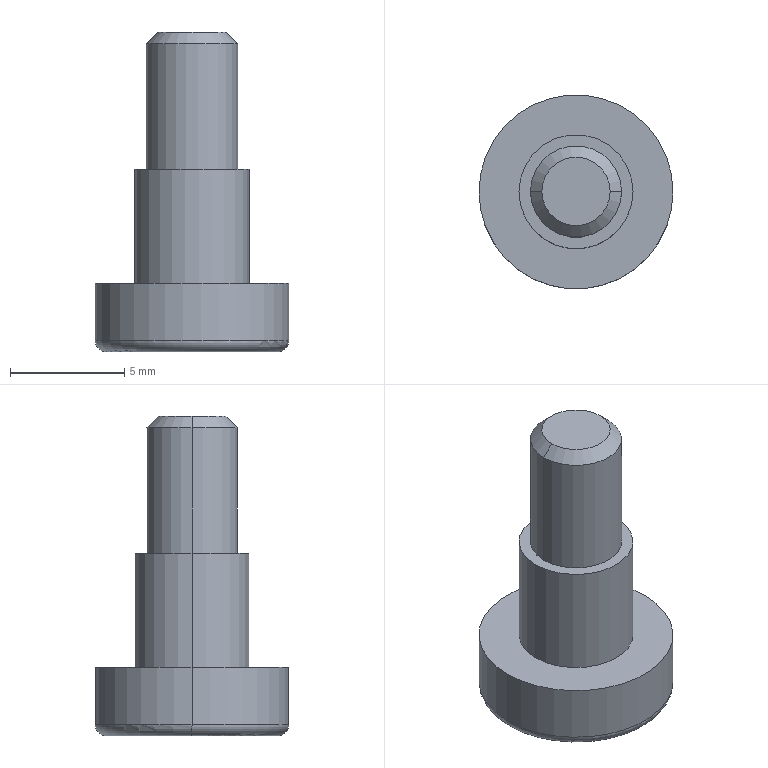Part | STEP file | 1 solid | 21 faces | box 8.5 x 8.5 x 14 mm | volume 317.59 mm3 | plane 11 | cylinder 6 | torus 2 | cone 2 | commonest cylinder face diameters 4 x2 5 x2 8.5 x2
STEP:
#1=CARTESIAN_POINT('',(0.,0.,0.));
#2=DIRECTION('',(0.,0.,1.));
#3=DIRECTION('',(1.,0.,0.));
#4=AXIS2_PLACEMENT_3D('',#1,#2,#3);
#5=CARTESIAN_POINT('',(-3.75,0.,0.));
#6=VERTEX_POINT('',#5);
#7=CARTESIAN_POINT('',(3.75,0.,0.));
#8=VERTEX_POINT('',#7);
#9=CARTESIAN_POINT('',(0.,0.,0.));
#10=DIRECTION('',(0.,0.,-1.));
#11=DIRECTION('',(1.,0.,0.));
#12=AXIS2_PLACEMENT_3D('',#9,#10,#11);
#13=CIRCLE('',#12,3.75);
#14=CARTESIAN_POINT('',(0.,0.,0.5));
#15=DIRECTION('',(0.,0.,1.));
#16=DIRECTION('',(1.,0.,0.));
#17=AXIS2_PLACEMENT_3D('',#14,#15,#16);
#18=TOROIDAL_SURFACE('',#17,3.75,0.5);
#19=CARTESIAN_POINT('',(6.283,4.712));
#20=DIRECTION('',(-1.,0.));
#21=VECTOR('',#20,1.);
#22=LINE('',#19,#21);
#23=(GEOMETRIC_REPRESENTATION_CONTEXT(2)PARAMETRIC_REPRESENTATION_CONTEXT()REPRESENTATION_CONTEXT('',''));
#24=DEFINITIONAL_REPRESENTATION('',(#22),#23);
#25=PCURVE('',#18,#24);
#26=CARTESIAN_POINT('',(0.,0.,0.));
#27=DIRECTION('',(0.,0.,1.));
#28=DIRECTION('',(1.,0.,0.));
#29=AXIS2_PLACEMENT_3D('',#26,#27,#28);
#30=PLANE('',#29);
#31=CARTESIAN_POINT('',(3.75,0.));
#32=CARTESIAN_POINT('',(3.75,-6.495));
#33=CARTESIAN_POINT('',(-1.875,-3.248));
#34=CARTESIAN_POINT('',(-7.5,0.));
#35=CARTESIAN_POINT('',(-1.875,3.248));
#36=CARTESIAN_POINT('',(3.75,6.495));
#37=CARTESIAN_POINT('',(3.75,0.));
#38=(BOUNDED_CURVE()B_SPLINE_CURVE(2,(#31,#32,#33,#34,#35,#36,#37),.UNSPECIFIED.,.T.,.F.)B_SPLINE_CURVE_WITH_KNOTS((1,2,2,2,2,1),(-2.094,0.,2.094,4.189,6.283,8.378),.UNSPECIFIED.)CURVE()GEOMETRIC_REPRESENTATION_ITEM()RATIONAL_B_SPLINE_CURVE((1.,0.5,1.,0.5,1.,0.5,1.))REPRESENTATION_ITEM(''));
#39=(GEOMETRIC_REPRESENTATION_CONTEXT(2)PARAMETRIC_REPRESENTATION_CONTEXT()REPRESENTATION_CONTEXT('',''));
#40=DEFINITIONAL_REPRESENTATION('',(#38),#39);
#41=PCURVE('',#30,#40);
#42=SURFACE_CURVE('',#13,(#25,#41),.PCURVE_S1.);
#43=EDGE_CURVE('',#6,#8,#42,.T.);
#44=ORIENTED_EDGE('',*,*,#43,.F.);
#45=CARTESIAN_POINT('',(-4.25,0.,0.5));
#46=VERTEX_POINT('',#45);
#47=CARTESIAN_POINT('',(-3.75,0.,0.5));
#48=DIRECTION('',(0.,1.,0.));
#49=DIRECTION('',(-1.,0.,0.));
#50=AXIS2_PLACEMENT_3D('',#47,#48,#49);
#51=CIRCLE('',#50,0.5);
#52=CARTESIAN_POINT('',(3.142,0.));
#53=DIRECTION('',(0.,1.));
#54=VECTOR('',#53,1.);
#55=LINE('',#52,#54);
#56=(GEOMETRIC_REPRESENTATION_CONTEXT(2)PARAMETRIC_REPRESENTATION_CONTEXT()REPRESENTATION_CONTEXT('',''));
#57=DEFINITIONAL_REPRESENTATION('',(#55),#56);
#58=PCURVE('',#18,#57);
#59=CARTESIAN_POINT('',(0.,0.,0.5));
#60=DIRECTION('',(0.,0.,1.));
#61=DIRECTION('',(1.,0.,0.));
#62=AXIS2_PLACEMENT_3D('',#59,#60,#61);
#63=TOROIDAL_SURFACE('',#62,3.75,0.5);
#64=CARTESIAN_POINT('',(3.142,0.));
#65=DIRECTION('',(0.,1.));
#66=VECTOR('',#65,1.);
#67=LINE('',#64,#66);
#68=(GEOMETRIC_REPRESENTATION_CONTEXT(2)PARAMETRIC_REPRESENTATION_CONTEXT()REPRESENTATION_CONTEXT('',''));
#69=DEFINITIONAL_REPRESENTATION('',(#67),#68);
#70=PCURVE('',#63,#69);
#71=SURFACE_CURVE('',#51,(#58,#70),.PCURVE_S1.);
#72=EDGE_CURVE('',#6,#46,#71,.T.);
#73=ORIENTED_EDGE('',*,*,#72,.T.);
#74=CARTESIAN_POINT('',(4.25,0.,0.5));
#75=VERTEX_POINT('',#74);
#76=CARTESIAN_POINT('',(0.,0.,0.5));
#77=DIRECTION('',(0.,0.,1.));
#78=DIRECTION('',(1.,0.,0.));
#79=AXIS2_PLACEMENT_3D('',#76,#77,#78);
#80=CIRCLE('',#79,4.25);
#81=CARTESIAN_POINT('',(0.,6.283));
#82=DIRECTION('',(1.,0.));
#83=VECTOR('',#82,1.);
#84=LINE('',#81,#83);
#85=(GEOMETRIC_REPRESENTATION_CONTEXT(2)PARAMETRIC_REPRESENTATION_CONTEXT()REPRESENTATION_CONTEXT('',''));
#86=DEFINITIONAL_REPRESENTATION('',(#84),#85);
#87=PCURVE('',#18,#86);
#88=CARTESIAN_POINT('',(0.,0.,3.));
#89=DIRECTION('',(0.,0.,-1.));
#90=DIRECTION('',(-1.,0.,0.));
#91=AXIS2_PLACEMENT_3D('',#88,#89,#90);
#92=CYLINDRICAL_SURFACE('',#91,4.25);
#93=CARTESIAN_POINT('',(3.142,2.5));
#94=DIRECTION('',(-1.,0.));
#95=VECTOR('',#94,1.);
#96=LINE('',#93,#95);
#97=(GEOMETRIC_REPRESENTATION_CONTEXT(2)PARAMETRIC_REPRESENTATION_CONTEXT()REPRESENTATION_CONTEXT('',''));
#98=DEFINITIONAL_REPRESENTATION('',(#96),#97);
#99=PCURVE('',#92,#98);
#100=SURFACE_CURVE('',#80,(#87,#99),.PCURVE_S1.);
#101=EDGE_CURVE('',#75,#46,#100,.T.);
#102=ORIENTED_EDGE('',*,*,#101,.F.);
#103=CARTESIAN_POINT('',(3.75,0.,0.5));
#104=DIRECTION('',(0.,-1.,0.));
#105=DIRECTION('',(0.,0.,-1.));
#106=AXIS2_PLACEMENT_3D('',#103,#104,#105);
#107=CIRCLE('',#106,0.5);
#108=CARTESIAN_POINT('',(0.,4.712));
#109=DIRECTION('',(0.,1.));
#110=VECTOR('',#109,1.);
#111=LINE('',#108,#110);
#112=(GEOMETRIC_REPRESENTATION_CONTEXT(2)PARAMETRIC_REPRESENTATION_CONTEXT()REPRESENTATION_CONTEXT('',''));
#113=DEFINITIONAL_REPRESENTATION('',(#111),#112);
#114=PCURVE('',#18,#113);
#115=CARTESIAN_POINT('',(6.283,4.712));
#116=DIRECTION('',(0.,1.));
#117=VECTOR('',#116,1.);
#118=LINE('',#115,#117);
#119=(GEOMETRIC_REPRESENTATION_CONTEXT(2)PARAMETRIC_REPRESENTATION_CONTEXT()REPRESENTATION_CONTEXT('',''));
#120=DEFINITIONAL_REPRESENTATION('',(#118),#119);
#121=PCURVE('',#63,#120);
#122=SURFACE_CURVE('',#107,(#114,#121),.PCURVE_S1.);
#123=EDGE_CURVE('',#8,#75,#122,.T.);
#124=ORIENTED_EDGE('',*,*,#123,.F.);
#125=EDGE_LOOP('',(#44,#73,#102,#124));
#126=FACE_BOUND('',#125,.T.);
#127=ADVANCED_FACE('',(#126),#18,.T.);
#128=CARTESIAN_POINT('',(1.5,0.,14.));
#129=VERTEX_POINT('',#128);
#130=CARTESIAN_POINT('',(-1.5,0.,14.));
#131=VERTEX_POINT('',#130);
#132=CARTESIAN_POINT('',(0.,0.,14.));
#133=DIRECTION('',(0.,0.,1.));
#134=DIRECTION('',(1.,0.,0.));
#135=AXIS2_PLACEMENT_3D('',#132,#133,#134);
#136=CIRCLE('',#135,1.5);
#137=CARTESIAN_POINT('',(0.,0.,14.));
#138=DIRECTION('',(0.,0.,-1.));
#139=DIRECTION('',(-1.,0.,0.));
#140=AXIS2_PLACEMENT_3D('',#137,#138,#139);
#141=CONICAL_SURFACE('',#140,1.5,0.7854);
#142=CARTESIAN_POINT('',(3.142,0.));
#143=DIRECTION('',(-1.,0.));
#144=VECTOR('',#143,1.);
#145=LINE('',#142,#144);
#146=(GEOMETRIC_REPRESENTATION_CONTEXT(2)PARAMETRIC_REPRESENTATION_CONTEXT()REPRESENTATION_CONTEXT('',''));
#147=DEFINITIONAL_REPRESENTATION('',(#145),#146);
#148=PCURVE('',#141,#147);
#149=CARTESIAN_POINT('',(0.,0.,14.));
#150=DIRECTION('',(0.,0.,1.));
#151=DIRECTION('',(1.,0.,0.));
#152=AXIS2_PLACEMENT_3D('',#149,#150,#151);
#153=PLANE('',#152);
#154=CARTESIAN_POINT('',(0.,0.));
#155=DIRECTION('',(1.,0.));
#156=AXIS2_PLACEMENT_2D('',#154,#155);
#157=CIRCLE('',#156,1.5);
#158=(GEOMETRIC_REPRESENTATION_CONTEXT(2)PARAMETRIC_REPRESENTATION_CONTEXT()REPRESENTATION_CONTEXT('',''));
#159=DEFINITIONAL_REPRESENTATION('',(#157),#158);
#160=PCURVE('',#153,#159);
#161=SURFACE_CURVE('',#136,(#148,#160),.PCURVE_S1.);
#162=EDGE_CURVE('',#129,#131,#161,.T.);
#163=ORIENTED_EDGE('',*,*,#162,.F.);
#164=CARTESIAN_POINT('',(2.,0.,13.5));
#165=VERTEX_POINT('',#164);
#166=CARTESIAN_POINT('',(1.5,0.,14.));
#167=DIRECTION('',(0.7071,0.,-0.7071));
#168=VECTOR('',#167,1.);
#169=LINE('',#166,#168);
#170=CARTESIAN_POINT('',(3.142,0.));
#171=DIRECTION('',(0.,1.));
#172=VECTOR('',#171,1.);
#173=LINE('',#170,#172);
#174=(GEOMETRIC_REPRESENTATION_CONTEXT(2)PARAMETRIC_REPRESENTATION_CONTEXT()REPRESENTATION_CONTEXT('',''));
#175=DEFINITIONAL_REPRESENTATION('',(#173),#174);
#176=PCURVE('',#141,#175);
#177=CARTESIAN_POINT('',(0.,0.,14.));
#178=DIRECTION('',(0.,0.,-1.));
#179=DIRECTION('',(-1.,0.,0.));
#180=AXIS2_PLACEMENT_3D('',#177,#178,#179);
#181=CONICAL_SURFACE('',#180,1.5,0.7854);
#182=CARTESIAN_POINT('',(3.142,0.));
#183=DIRECTION('',(0.,1.));
#184=VECTOR('',#183,1.);
#185=LINE('',#182,#184);
#186=(GEOMETRIC_REPRESENTATION_CONTEXT(2)PARAMETRIC_REPRESENTATION_CONTEXT()REPRESENTATION_CONTEXT('',''));
#187=DEFINITIONAL_REPRESENTATION('',(#185),#186);
#188=PCURVE('',#181,#187);
#189=SURFACE_CURVE('',#169,(#176,#188),.PCURVE_S1.);
#190=EDGE_CURVE('',#129,#165,#189,.T.);
#191=ORIENTED_EDGE('',*,*,#190,.T.);
#192=CARTESIAN_POINT('',(-2.,0.,13.5));
#193=VERTEX_POINT('',#192);
#194=CARTESIAN_POINT('',(0.,0.,13.5));
#195=DIRECTION('',(0.,0.,-1.));
#196=DIRECTION('',(1.,0.,0.));
#197=AXIS2_PLACEMENT_3D('',#194,#195,#196);
#198=CIRCLE('',#197,2.);
#199=CARTESIAN_POINT('',(-3.142,0.5));
#200=DIRECTION('',(1.,0.));
#201=VECTOR('',#200,1.);
#202=LINE('',#199,#201);
#203=(GEOMETRIC_REPRESENTATION_CONTEXT(2)PARAMETRIC_REPRESENTATION_CONTEXT()REPRESENTATION_CONTEXT('',''));
#204=DEFINITIONAL_REPRESENTATION('',(#202),#203);
#205=PCURVE('',#141,#204);
#206=CARTESIAN_POINT('',(0.,0.,14.));
#207=DIRECTION('',(0.,0.,-1.));
#208=DIRECTION('',(-1.,0.,0.));
#209=AXIS2_PLACEMENT_3D('',#206,#207,#208);
#210=CYLINDRICAL_SURFACE('',#209,2.);
#211=CARTESIAN_POINT('',(-3.142,0.5));
#212=DIRECTION('',(1.,0.));
#213=VECTOR('',#212,1.);
#214=LINE('',#211,#213);
#215=(GEOMETRIC_REPRESENTATION_CONTEXT(2)PARAMETRIC_REPRESENTATION_CONTEXT()REPRESENTATION_CONTEXT('',''));
#216=DEFINITIONAL_REPRESENTATION('',(#214),#215);
#217=PCURVE('',#210,#216);
#218=SURFACE_CURVE('',#198,(#205,#217),.PCURVE_S1.);
#219=EDGE_CURVE('',#193,#165,#218,.T.);
#220=ORIENTED_EDGE('',*,*,#219,.F.);
#221=CARTESIAN_POINT('',(-1.5,0.,14.));
#222=DIRECTION('',(-0.7071,0.,-0.7071));
#223=VECTOR('',#222,1.);
#224=LINE('',#221,#223);
#225=CARTESIAN_POINT('',(0.,0.));
#226=DIRECTION('',(0.,1.));
#227=VECTOR('',#226,1.);
#228=LINE('',#225,#227);
#229=(GEOMETRIC_REPRESENTATION_CONTEXT(2)PARAMETRIC_REPRESENTATION_CONTEXT()REPRESENTATION_CONTEXT('',''));
#230=DEFINITIONAL_REPRESENTATION('',(#228),#229);
#231=PCURVE('',#141,#230);
#232=CARTESIAN_POINT('',(6.283,0.));
#233=DIRECTION('',(0.,1.));
#234=VECTOR('',#233,1.);
#235=LINE('',#232,#234);
#236=(GEOMETRIC_REPRESENTATION_CONTEXT(2)PARAMETRIC_REPRESENTATION_CONTEXT()REPRESENTATION_CONTEXT('',''));
#237=DEFINITIONAL_REPRESENTATION('',(#235),#236);
#238=PCURVE('',#181,#237);
#239=SURFACE_CURVE('',#224,(#231,#238),.PCURVE_S1.);
#240=EDGE_CURVE('',#131,#193,#239,.T.);
#241=ORIENTED_EDGE('',*,*,#240,.F.);
#242=EDGE_LOOP('',(#163,#191,#220,#241));
#243=FACE_BOUND('',#242,.T.);
#244=ADVANCED_FACE('',(#243),#141,.T.);
#245=ORIENTED_EDGE('',*,*,#219,.T.);
#246=CARTESIAN_POINT('',(2.,0.,8.));
#247=VERTEX_POINT('',#246);
#248=CARTESIAN_POINT('',(2.,0.,14.));
#249=DIRECTION('',(0.,0.,-1.));
#250=VECTOR('',#249,1.);
#251=LINE('',#248,#250);
#252=CARTESIAN_POINT('',(3.142,0.));
#253=DIRECTION('',(0.,1.));
#254=VECTOR('',#253,1.);
#255=LINE('',#252,#254);
#256=(GEOMETRIC_REPRESENTATION_CONTEXT(2)PARAMETRIC_REPRESENTATION_CONTEXT()REPRESENTATION_CONTEXT('',''));
#257=DEFINITIONAL_REPRESENTATION('',(#255),#256);
#258=PCURVE('',#210,#257);
#259=CARTESIAN_POINT('',(0.,0.,14.));
#260=DIRECTION('',(0.,0.,-1.));
#261=DIRECTION('',(-1.,0.,0.));
#262=AXIS2_PLACEMENT_3D('',#259,#260,#261);
#263=CYLINDRICAL_SURFACE('',#262,2.);
#264=CARTESIAN_POINT('',(3.142,0.));
#265=DIRECTION('',(0.,1.));
#266=VECTOR('',#265,1.);
#267=LINE('',#264,#266);
#268=(GEOMETRIC_REPRESENTATION_CONTEXT(2)PARAMETRIC_REPRESENTATION_CONTEXT()REPRESENTATION_CONTEXT('',''));
#269=DEFINITIONAL_REPRESENTATION('',(#267),#268);
#270=PCURVE('',#263,#269);
#271=SURFACE_CURVE('',#251,(#258,#270),.PCURVE_S1.);
#272=EDGE_CURVE('',#165,#247,#271,.T.);
#273=ORIENTED_EDGE('',*,*,#272,.T.);
#274=CARTESIAN_POINT('',(-2.,0.,8.));
#275=VERTEX_POINT('',#274);
#276=CARTESIAN_POINT('',(0.,0.,8.));
#277=DIRECTION('',(0.,0.,1.));
#278=DIRECTION('',(1.,0.,0.));
#279=AXIS2_PLACEMENT_3D('',#276,#277,#278);
#280=CIRCLE('',#279,2.);
#281=CARTESIAN_POINT('',(3.142,6.));
#282=DIRECTION('',(-1.,0.));
#283=VECTOR('',#282,1.);
#284=LINE('',#281,#283);
#285=(GEOMETRIC_REPRESENTATION_CONTEXT(2)PARAMETRIC_REPRESENTATION_CONTEXT()REPRESENTATION_CONTEXT('',''));
#286=DEFINITIONAL_REPRESENTATION('',(#284),#285);
#287=PCURVE('',#210,#286);
#288=CARTESIAN_POINT('',(0.,0.,8.));
#289=DIRECTION('',(0.,0.,1.));
#290=DIRECTION('',(1.,0.,0.));
#291=AXIS2_PLACEMENT_3D('',#288,#289,#290);
#292=PLANE('',#291);
#293=CARTESIAN_POINT('',(0.,0.));
#294=DIRECTION('',(1.,0.));
#295=AXIS2_PLACEMENT_2D('',#293,#294);
#296=CIRCLE('',#295,2.);
#297=(GEOMETRIC_REPRESENTATION_CONTEXT(2)PARAMETRIC_REPRESENTATION_CONTEXT()REPRESENTATION_CONTEXT('',''));
#298=DEFINITIONAL_REPRESENTATION('',(#296),#297);
#299=PCURVE('',#292,#298);
#300=SURFACE_CURVE('',#280,(#287,#299),.PCURVE_S1.);
#301=EDGE_CURVE('',#247,#275,#300,.T.);
#302=ORIENTED_EDGE('',*,*,#301,.T.);
#303=CARTESIAN_POINT('',(-2.,0.,14.));
#304=DIRECTION('',(0.,0.,-1.));
#305=VECTOR('',#304,1.);
#306=LINE('',#303,#305);
#307=CARTESIAN_POINT('',(0.,0.));
#308=DIRECTION('',(0.,1.));
#309=VECTOR('',#308,1.);
#310=LINE('',#307,#309);
#311=(GEOMETRIC_REPRESENTATION_CONTEXT(2)PARAMETRIC_REPRESENTATION_CONTEXT()REPRESENTATION_CONTEXT('',''));
#312=DEFINITIONAL_REPRESENTATION('',(#310),#311);
#313=PCURVE('',#210,#312);
#314=CARTESIAN_POINT('',(6.283,0.));
#315=DIRECTION('',(0.,1.));
#316=VECTOR('',#315,1.);
#317=LINE('',#314,#316);
#318=(GEOMETRIC_REPRESENTATION_CONTEXT(2)PARAMETRIC_REPRESENTATION_CONTEXT()REPRESENTATION_CONTEXT('',''));
#319=DEFINITIONAL_REPRESENTATION('',(#317),#318);
#320=PCURVE('',#263,#319);
#321=SURFACE_CURVE('',#306,(#313,#320),.PCURVE_S1.);
#322=EDGE_CURVE('',#193,#275,#321,.T.);
#323=ORIENTED_EDGE('',*,*,#322,.F.);
#324=EDGE_LOOP('',(#245,#273,#302,#323));
#325=FACE_BOUND('',#324,.T.);
#326=ADVANCED_FACE('',(#325),#210,.T.);
#327=CARTESIAN_POINT('',(2.5,0.,8.));
#328=VERTEX_POINT('',#327);
#329=CARTESIAN_POINT('',(-2.5,0.,8.));
#330=VERTEX_POINT('',#329);
#331=CARTESIAN_POINT('',(0.,0.,8.));
#332=DIRECTION('',(0.,0.,1.));
#333=DIRECTION('',(1.,0.,0.));
#334=AXIS2_PLACEMENT_3D('',#331,#332,#333);
#335=CIRCLE('',#334,2.5);
#336=CARTESIAN_POINT('',(0.,0.,8.));
#337=DIRECTION('',(0.,0.,-1.));
#338=DIRECTION('',(-1.,0.,0.));
#339=AXIS2_PLACEMENT_3D('',#336,#337,#338);
#340=CYLINDRICAL_SURFACE('',#339,2.5);
#341=CARTESIAN_POINT('',(3.142,0.));
#342=DIRECTION('',(-1.,0.));
#343=VECTOR('',#342,1.);
#344=LINE('',#341,#343);
#345=(GEOMETRIC_REPRESENTATION_CONTEXT(2)PARAMETRIC_REPRESENTATION_CONTEXT()REPRESENTATION_CONTEXT('',''));
#346=DEFINITIONAL_REPRESENTATION('',(#344),#345);
#347=PCURVE('',#340,#346);
#348=CARTESIAN_POINT('',(0.,0.));
#349=DIRECTION('',(1.,0.));
#350=AXIS2_PLACEMENT_2D('',#348,#349);
#351=CIRCLE('',#350,2.5);
#352=(GEOMETRIC_REPRESENTATION_CONTEXT(2)PARAMETRIC_REPRESENTATION_CONTEXT()REPRESENTATION_CONTEXT('',''));
#353=DEFINITIONAL_REPRESENTATION('',(#351),#352);
#354=PCURVE('',#292,#353);
#355=SURFACE_CURVE('',#335,(#347,#354),.PCURVE_S1.);
#356=EDGE_CURVE('',#328,#330,#355,.T.);
#357=ORIENTED_EDGE('',*,*,#356,.F.);
#358=CARTESIAN_POINT('',(2.5,0.,3.));
#359=VERTEX_POINT('',#358);
#360=CARTESIAN_POINT('',(2.5,0.,8.));
#361=DIRECTION('',(0.,0.,-1.));
#362=VECTOR('',#361,1.);
#363=LINE('',#360,#362);
#364=CARTESIAN_POINT('',(3.142,0.));
#365=DIRECTION('',(0.,1.));
#366=VECTOR('',#365,1.);
#367=LINE('',#364,#366);
#368=(GEOMETRIC_REPRESENTATION_CONTEXT(2)PARAMETRIC_REPRESENTATION_CONTEXT()REPRESENTATION_CONTEXT('',''));
#369=DEFINITIONAL_REPRESENTATION('',(#367),#368);
#370=PCURVE('',#340,#369);
#371=CARTESIAN_POINT('',(0.,0.,8.));
#372=DIRECTION('',(0.,0.,-1.));
#373=DIRECTION('',(-1.,0.,0.));
#374=AXIS2_PLACEMENT_3D('',#371,#372,#373);
#375=CYLINDRICAL_SURFACE('',#374,2.5);
#376=CARTESIAN_POINT('',(3.142,0.));
#377=DIRECTION('',(0.,1.));
#378=VECTOR('',#377,1.);
#379=LINE('',#376,#378);
#380=(GEOMETRIC_REPRESENTATION_CONTEXT(2)PARAMETRIC_REPRESENTATION_CONTEXT()REPRESENTATION_CONTEXT('',''));
#381=DEFINITIONAL_REPRESENTATION('',(#379),#380);
#382=PCURVE('',#375,#381);
#383=SURFACE_CURVE('',#363,(#370,#382),.PCURVE_S1.);
#384=EDGE_CURVE('',#328,#359,#383,.T.);
#385=ORIENTED_EDGE('',*,*,#384,.T.);
#386=CARTESIAN_POINT('',(-2.5,0.,3.));
#387=VERTEX_POINT('',#386);
#388=CARTESIAN_POINT('',(0.,0.,3.));
#389=DIRECTION('',(0.,0.,1.));
#390=DIRECTION('',(1.,0.,0.));
#391=AXIS2_PLACEMENT_3D('',#388,#389,#390);
#392=CIRCLE('',#391,2.5);
#393=CARTESIAN_POINT('',(3.142,5.));
#394=DIRECTION('',(-1.,0.));
#395=VECTOR('',#394,1.);
#396=LINE('',#393,#395);
#397=(GEOMETRIC_REPRESENTATION_CONTEXT(2)PARAMETRIC_REPRESENTATION_CONTEXT()REPRESENTATION_CONTEXT('',''));
#398=DEFINITIONAL_REPRESENTATION('',(#396),#397);
#399=PCURVE('',#340,#398);
#400=CARTESIAN_POINT('',(0.,0.,3.));
#401=DIRECTION('',(0.,0.,1.));
#402=DIRECTION('',(1.,0.,0.));
#403=AXIS2_PLACEMENT_3D('',#400,#401,#402);
#404=PLANE('',#403);
#405=CARTESIAN_POINT('',(0.,0.));
#406=DIRECTION('',(1.,0.));
#407=AXIS2_PLACEMENT_2D('',#405,#406);
#408=CIRCLE('',#407,2.5);
#409=(GEOMETRIC_REPRESENTATION_CONTEXT(2)PARAMETRIC_REPRESENTATION_CONTEXT()REPRESENTATION_CONTEXT('',''));
#410=DEFINITIONAL_REPRESENTATION('',(#408),#409);
#411=PCURVE('',#404,#410);
#412=SURFACE_CURVE('',#392,(#399,#411),.PCURVE_S1.);
#413=EDGE_CURVE('',#359,#387,#412,.T.);
#414=ORIENTED_EDGE('',*,*,#413,.T.);
#415=CARTESIAN_POINT('',(-2.5,0.,8.));
#416=DIRECTION('',(0.,0.,-1.));
#417=VECTOR('',#416,1.);
#418=LINE('',#415,#417);
#419=CARTESIAN_POINT('',(0.,0.));
#420=DIRECTION('',(0.,1.));
#421=VECTOR('',#420,1.);
#422=LINE('',#419,#421);
#423=(GEOMETRIC_REPRESENTATION_CONTEXT(2)PARAMETRIC_REPRESENTATION_CONTEXT()REPRESENTATION_CONTEXT('',''));
#424=DEFINITIONAL_REPRESENTATION('',(#422),#423);
#425=PCURVE('',#340,#424);
#426=CARTESIAN_POINT('',(6.283,0.));
#427=DIRECTION('',(0.,1.));
#428=VECTOR('',#427,1.);
#429=LINE('',#426,#428);
#430=(GEOMETRIC_REPRESENTATION_CONTEXT(2)PARAMETRIC_REPRESENTATION_CONTEXT()REPRESENTATION_CONTEXT('',''));
#431=DEFINITIONAL_REPRESENTATION('',(#429),#430);
#432=PCURVE('',#375,#431);
#433=SURFACE_CURVE('',#418,(#425,#432),.PCURVE_S1.);
#434=EDGE_CURVE('',#330,#387,#433,.T.);
#435=ORIENTED_EDGE('',*,*,#434,.F.);
#436=EDGE_LOOP('',(#357,#385,#414,#435));
#437=FACE_BOUND('',#436,.T.);
#438=ADVANCED_FACE('',(#437),#340,.T.);
#439=CARTESIAN_POINT('',(4.25,0.,3.));
#440=VERTEX_POINT('',#439);
#441=CARTESIAN_POINT('',(-4.25,0.,3.));
#442=VERTEX_POINT('',#441);
#443=CARTESIAN_POINT('',(0.,0.,3.));
#444=DIRECTION('',(0.,0.,1.));
#445=DIRECTION('',(1.,0.,0.));
#446=AXIS2_PLACEMENT_3D('',#443,#444,#445);
#447=CIRCLE('',#446,4.25);
#448=CARTESIAN_POINT('',(3.142,0.));
#449=DIRECTION('',(-1.,0.));
#450=VECTOR('',#449,1.);
#451=LINE('',#448,#450);
#452=(GEOMETRIC_REPRESENTATION_CONTEXT(2)PARAMETRIC_REPRESENTATION_CONTEXT()REPRESENTATION_CONTEXT('',''));
#453=DEFINITIONAL_REPRESENTATION('',(#451),#452);
#454=PCURVE('',#92,#453);
#455=CARTESIAN_POINT('',(0.,0.));
#456=DIRECTION('',(1.,0.));
#457=AXIS2_PLACEMENT_2D('',#455,#456);
#458=CIRCLE('',#457,4.25);
#459=(GEOMETRIC_REPRESENTATION_CONTEXT(2)PARAMETRIC_REPRESENTATION_CONTEXT()REPRESENTATION_CONTEXT('',''));
#460=DEFINITIONAL_REPRESENTATION('',(#458),#459);
#461=PCURVE('',#404,#460);
#462=SURFACE_CURVE('',#447,(#454,#461),.PCURVE_S1.);
#463=EDGE_CURVE('',#440,#442,#462,.T.);
#464=ORIENTED_EDGE('',*,*,#463,.F.);
#465=CARTESIAN_POINT('',(4.25,0.,3.));
#466=DIRECTION('',(0.,0.,-1.));
#467=VECTOR('',#466,1.);
#468=LINE('',#465,#467);
#469=CARTESIAN_POINT('',(3.142,0.));
#470=DIRECTION('',(0.,1.));
#471=VECTOR('',#470,1.);
#472=LINE('',#469,#471);
#473=(GEOMETRIC_REPRESENTATION_CONTEXT(2)PARAMETRIC_REPRESENTATION_CONTEXT()REPRESENTATION_CONTEXT('',''));
#474=DEFINITIONAL_REPRESENTATION('',(#472),#473);
#475=PCURVE('',#92,#474);
#476=CARTESIAN_POINT('',(0.,0.,3.));
#477=DIRECTION('',(0.,0.,-1.));
#478=DIRECTION('',(-1.,0.,0.));
#479=AXIS2_PLACEMENT_3D('',#476,#477,#478);
#480=CYLINDRICAL_SURFACE('',#479,4.25);
#481=CARTESIAN_POINT('',(3.142,0.));
#482=DIRECTION('',(0.,1.));
#483=VECTOR('',#482,1.);
#484=LINE('',#481,#483);
#485=(GEOMETRIC_REPRESENTATION_CONTEXT(2)PARAMETRIC_REPRESENTATION_CONTEXT()REPRESENTATION_CONTEXT('',''));
#486=DEFINITIONAL_REPRESENTATION('',(#484),#485);
#487=PCURVE('',#480,#486);
#488=SURFACE_CURVE('',#468,(#475,#487),.PCURVE_S1.);
#489=EDGE_CURVE('',#440,#75,#488,.T.);
#490=ORIENTED_EDGE('',*,*,#489,.T.);
#491=ORIENTED_EDGE('',*,*,#101,.T.);
#492=CARTESIAN_POINT('',(-4.25,0.,3.));
#493=DIRECTION('',(0.,0.,-1.));
#494=VECTOR('',#493,1.);
#495=LINE('',#492,#494);
#496=CARTESIAN_POINT('',(0.,0.));
#497=DIRECTION('',(0.,1.));
#498=VECTOR('',#497,1.);
#499=LINE('',#496,#498);
#500=(GEOMETRIC_REPRESENTATION_CONTEXT(2)PARAMETRIC_REPRESENTATION_CONTEXT()REPRESENTATION_CONTEXT('',''));
#501=DEFINITIONAL_REPRESENTATION('',(#499),#500);
#502=PCURVE('',#92,#501);
#503=CARTESIAN_POINT('',(6.283,0.));
#504=DIRECTION('',(0.,1.));
#505=VECTOR('',#504,1.);
#506=LINE('',#503,#505);
#507=(GEOMETRIC_REPRESENTATION_CONTEXT(2)PARAMETRIC_REPRESENTATION_CONTEXT()REPRESENTATION_CONTEXT('',''));
#508=DEFINITIONAL_REPRESENTATION('',(#506),#507);
#509=PCURVE('',#480,#508);
#510=SURFACE_CURVE('',#495,(#502,#509),.PCURVE_S1.);
#511=EDGE_CURVE('',#442,#46,#510,.T.);
#512=ORIENTED_EDGE('',*,*,#511,.F.);
#513=EDGE_LOOP('',(#464,#490,#491,#512));
#514=FACE_BOUND('',#513,.T.);
#515=ADVANCED_FACE('',(#514),#92,.T.);
#516=ORIENTED_EDGE('',*,*,#489,.F.);
#517=CARTESIAN_POINT('',(0.,0.,3.));
#518=DIRECTION('',(0.,0.,1.));
#519=DIRECTION('',(1.,0.,0.));
#520=AXIS2_PLACEMENT_3D('',#517,#518,#519);
#521=CIRCLE('',#520,4.25);
#522=CARTESIAN_POINT('',(9.425,0.));
#523=DIRECTION('',(-1.,0.));
#524=VECTOR('',#523,1.);
#525=LINE('',#522,#524);
#526=(GEOMETRIC_REPRESENTATION_CONTEXT(2)PARAMETRIC_REPRESENTATION_CONTEXT()REPRESENTATION_CONTEXT('',''));
#527=DEFINITIONAL_REPRESENTATION('',(#525),#526);
#528=PCURVE('',#480,#527);
#529=CARTESIAN_POINT('',(0.,0.));
#530=DIRECTION('',(1.,0.));
#531=AXIS2_PLACEMENT_2D('',#529,#530);
#532=CIRCLE('',#531,4.25);
#533=(GEOMETRIC_REPRESENTATION_CONTEXT(2)PARAMETRIC_REPRESENTATION_CONTEXT()REPRESENTATION_CONTEXT('',''));
#534=DEFINITIONAL_REPRESENTATION('',(#532),#533);
#535=PCURVE('',#404,#534);
#536=SURFACE_CURVE('',#521,(#528,#535),.PCURVE_S1.);
#537=EDGE_CURVE('',#442,#440,#536,.T.);
#538=ORIENTED_EDGE('',*,*,#537,.F.);
#539=ORIENTED_EDGE('',*,*,#511,.T.);
#540=CARTESIAN_POINT('',(0.,0.,0.5));
#541=DIRECTION('',(0.,0.,1.));
#542=DIRECTION('',(1.,0.,0.));
#543=AXIS2_PLACEMENT_3D('',#540,#541,#542);
#544=CIRCLE('',#543,4.25);
#545=CARTESIAN_POINT('',(9.425,2.5));
#546=DIRECTION('',(-1.,0.));
#547=VECTOR('',#546,1.);
#548=LINE('',#545,#547);
#549=(GEOMETRIC_REPRESENTATION_CONTEXT(2)PARAMETRIC_REPRESENTATION_CONTEXT()REPRESENTATION_CONTEXT('',''));
#550=DEFINITIONAL_REPRESENTATION('',(#548),#549);
#551=PCURVE('',#480,#550);
#552=CARTESIAN_POINT('',(0.,6.283));
#553=DIRECTION('',(1.,0.));
#554=VECTOR('',#553,1.);
#555=LINE('',#552,#554);
#556=(GEOMETRIC_REPRESENTATION_CONTEXT(2)PARAMETRIC_REPRESENTATION_CONTEXT()REPRESENTATION_CONTEXT('',''));
#557=DEFINITIONAL_REPRESENTATION('',(#555),#556);
#558=PCURVE('',#63,#557);
#559=SURFACE_CURVE('',#544,(#551,#558),.PCURVE_S1.);
#560=EDGE_CURVE('',#46,#75,#559,.T.);
#561=ORIENTED_EDGE('',*,*,#560,.T.);
#562=EDGE_LOOP('',(#516,#538,#539,#561));
#563=FACE_BOUND('',#562,.T.);
#564=ADVANCED_FACE('',(#563),#480,.T.);
#565=CARTESIAN_POINT('',(0.,0.,3.));
#566=DIRECTION('',(0.,0.,1.));
#567=DIRECTION('',(1.,0.,0.));
#568=AXIS2_PLACEMENT_3D('',#565,#566,#567);
#569=CIRCLE('',#568,2.5);
#570=CARTESIAN_POINT('',(0.,0.));
#571=DIRECTION('',(1.,0.));
#572=AXIS2_PLACEMENT_2D('',#570,#571);
#573=CIRCLE('',#572,2.5);
#574=(GEOMETRIC_REPRESENTATION_CONTEXT(2)PARAMETRIC_REPRESENTATION_CONTEXT()REPRESENTATION_CONTEXT('',''));
#575=DEFINITIONAL_REPRESENTATION('',(#573),#574);
#576=PCURVE('',#404,#575);
#577=CARTESIAN_POINT('',(9.425,5.));
#578=DIRECTION('',(-1.,0.));
#579=VECTOR('',#578,1.);
#580=LINE('',#577,#579);
#581=(GEOMETRIC_REPRESENTATION_CONTEXT(2)PARAMETRIC_REPRESENTATION_CONTEXT()REPRESENTATION_CONTEXT('',''));
#582=DEFINITIONAL_REPRESENTATION('',(#580),#581);
#583=PCURVE('',#375,#582);
#584=SURFACE_CURVE('',#569,(#576,#583),.PCURVE_S1.);
#585=EDGE_CURVE('',#387,#359,#584,.T.);
#586=ORIENTED_EDGE('',*,*,#585,.F.);
#587=ORIENTED_EDGE('',*,*,#413,.F.);
#588=EDGE_LOOP('',(#586,#587));
#589=FACE_BOUND('',#588,.T.);
#590=ORIENTED_EDGE('',*,*,#537,.T.);
#591=ORIENTED_EDGE('',*,*,#463,.T.);
#592=EDGE_LOOP('',(#590,#591));
#593=FACE_BOUND('',#592,.T.);
#594=ADVANCED_FACE('',(#589,#593),#404,.T.);
#595=CARTESIAN_POINT('',(-1.732,0.,0.));
#596=VERTEX_POINT('',#595);
#597=CARTESIAN_POINT('',(-0.866,1.5,0.));
#598=VERTEX_POINT('',#597);
#599=CARTESIAN_POINT('',(-1.732,0.,0.));
#600=DIRECTION('',(0.5,0.866,0.));
#601=VECTOR('',#600,1.);
#602=LINE('',#599,#601);
#603=CARTESIAN_POINT('',(-1.732,0.));
#604=DIRECTION('',(0.5,0.866));
#605=VECTOR('',#604,1.);
#606=LINE('',#603,#605);
#607=(GEOMETRIC_REPRESENTATION_CONTEXT(2)PARAMETRIC_REPRESENTATION_CONTEXT()REPRESENTATION_CONTEXT('',''));
#608=DEFINITIONAL_REPRESENTATION('',(#606),#607);
#609=PCURVE('',#30,#608);
#610=CARTESIAN_POINT('',(-1.732,0.,3.));
#611=DIRECTION('',(-0.866,0.5,0.));
#612=DIRECTION('',(-0.5,-0.866,0.));
#613=AXIS2_PLACEMENT_3D('',#610,#611,#612);
#614=PLANE('',#613);
#615=CARTESIAN_POINT('',(0.,-3.));
#616=DIRECTION('',(-1.,0.));
#617=VECTOR('',#616,1.);
#618=LINE('',#615,#617);
#619=(GEOMETRIC_REPRESENTATION_CONTEXT(2)PARAMETRIC_REPRESENTATION_CONTEXT()REPRESENTATION_CONTEXT('',''));
#620=DEFINITIONAL_REPRESENTATION('',(#618),#619);
#621=PCURVE('',#614,#620);
#622=SURFACE_CURVE('',#602,(#609,#621),.PCURVE_S1.);
#623=EDGE_CURVE('',#596,#598,#622,.T.);
#624=ORIENTED_EDGE('',*,*,#623,.F.);
#625=CARTESIAN_POINT('',(-0.866,-1.5,0.));
#626=VERTEX_POINT('',#625);
#627=CARTESIAN_POINT('',(-0.866,-1.5,0.));
#628=DIRECTION('',(-0.5,0.866,0.));
#629=VECTOR('',#628,1.);
#630=LINE('',#627,#629);
#631=CARTESIAN_POINT('',(-0.866,-1.5));
#632=DIRECTION('',(-0.5,0.866));
#633=VECTOR('',#632,1.);
#634=LINE('',#631,#633);
#635=(GEOMETRIC_REPRESENTATION_CONTEXT(2)PARAMETRIC_REPRESENTATION_CONTEXT()REPRESENTATION_CONTEXT('',''));
#636=DEFINITIONAL_REPRESENTATION('',(#634),#635);
#637=PCURVE('',#30,#636);
#638=CARTESIAN_POINT('',(-0.866,-1.5,3.));
#639=DIRECTION('',(-0.866,-0.5,0.));
#640=DIRECTION('',(0.5,-0.866,0.));
#641=AXIS2_PLACEMENT_3D('',#638,#639,#640);
#642=PLANE('',#641);
#643=CARTESIAN_POINT('',(0.,-3.));
#644=DIRECTION('',(-1.,0.));
#645=VECTOR('',#644,1.);
#646=LINE('',#643,#645);
#647=(GEOMETRIC_REPRESENTATION_CONTEXT(2)PARAMETRIC_REPRESENTATION_CONTEXT()REPRESENTATION_CONTEXT('',''));
#648=DEFINITIONAL_REPRESENTATION('',(#646),#647);
#649=PCURVE('',#642,#648);
#650=SURFACE_CURVE('',#630,(#637,#649),.PCURVE_S1.);
#651=EDGE_CURVE('',#626,#596,#650,.T.);
#652=ORIENTED_EDGE('',*,*,#651,.F.);
#653=CARTESIAN_POINT('',(0.866,-1.5,0.));
#654=VERTEX_POINT('',#653);
#655=CARTESIAN_POINT('',(0.866,-1.5,0.));
#656=DIRECTION('',(-1.,0.,0.));
#657=VECTOR('',#656,1.);
#658=LINE('',#655,#657);
#659=CARTESIAN_POINT('',(0.866,-1.5));
#660=DIRECTION('',(-1.,0.));
#661=VECTOR('',#660,1.);
#662=LINE('',#659,#661);
#663=(GEOMETRIC_REPRESENTATION_CONTEXT(2)PARAMETRIC_REPRESENTATION_CONTEXT()REPRESENTATION_CONTEXT('',''));
#664=DEFINITIONAL_REPRESENTATION('',(#662),#663);
#665=PCURVE('',#30,#664);
#666=CARTESIAN_POINT('',(0.866,-1.5,3.));
#667=DIRECTION('',(0.,-1.,0.));
#668=DIRECTION('',(0.,0.,-1.));
#669=AXIS2_PLACEMENT_3D('',#666,#667,#668);
#670=PLANE('',#669);
#671=CARTESIAN_POINT('',(3.,0.));
#672=DIRECTION('',(0.,-1.));
#673=VECTOR('',#672,1.);
#674=LINE('',#671,#673);
#675=(GEOMETRIC_REPRESENTATION_CONTEXT(2)PARAMETRIC_REPRESENTATION_CONTEXT()REPRESENTATION_CONTEXT('',''));
#676=DEFINITIONAL_REPRESENTATION('',(#674),#675);
#677=PCURVE('',#670,#676);
#678=SURFACE_CURVE('',#658,(#665,#677),.PCURVE_S1.);
#679=EDGE_CURVE('',#654,#626,#678,.T.);
#680=ORIENTED_EDGE('',*,*,#679,.F.);
#681=CARTESIAN_POINT('',(1.732,0.,0.));
#682=VERTEX_POINT('',#681);
#683=CARTESIAN_POINT('',(1.732,0.,0.));
#684=DIRECTION('',(-0.5,-0.866,0.));
#685=VECTOR('',#684,1.);
#686=LINE('',#683,#685);
#687=CARTESIAN_POINT('',(1.732,0.));
#688=DIRECTION('',(-0.5,-0.866));
#689=VECTOR('',#688,1.);
#690=LINE('',#687,#689);
#691=(GEOMETRIC_REPRESENTATION_CONTEXT(2)PARAMETRIC_REPRESENTATION_CONTEXT()REPRESENTATION_CONTEXT('',''));
#692=DEFINITIONAL_REPRESENTATION('',(#690),#691);
#693=PCURVE('',#30,#692);
#694=CARTESIAN_POINT('',(1.732,0.,3.));
#695=DIRECTION('',(0.866,-0.5,0.));
#696=DIRECTION('',(0.5,0.866,0.));
#697=AXIS2_PLACEMENT_3D('',#694,#695,#696);
#698=PLANE('',#697);
#699=CARTESIAN_POINT('',(0.,-3.));
#700=DIRECTION('',(-1.,0.));
#701=VECTOR('',#700,1.);
#702=LINE('',#699,#701);
#703=(GEOMETRIC_REPRESENTATION_CONTEXT(2)PARAMETRIC_REPRESENTATION_CONTEXT()REPRESENTATION_CONTEXT('',''));
#704=DEFINITIONAL_REPRESENTATION('',(#702),#703);
#705=PCURVE('',#698,#704);
#706=SURFACE_CURVE('',#686,(#693,#705),.PCURVE_S1.);
#707=EDGE_CURVE('',#682,#654,#706,.T.);
#708=ORIENTED_EDGE('',*,*,#707,.F.);
#709=CARTESIAN_POINT('',(0.866,1.5,0.));
#710=VERTEX_POINT('',#709);
#711=CARTESIAN_POINT('',(0.866,1.5,0.));
#712=DIRECTION('',(0.5,-0.866,0.));
#713=VECTOR('',#712,1.);
#714=LINE('',#711,#713);
#715=CARTESIAN_POINT('',(0.866,1.5));
#716=DIRECTION('',(0.5,-0.866));
#717=VECTOR('',#716,1.);
#718=LINE('',#715,#717);
#719=(GEOMETRIC_REPRESENTATION_CONTEXT(2)PARAMETRIC_REPRESENTATION_CONTEXT()REPRESENTATION_CONTEXT('',''));
#720=DEFINITIONAL_REPRESENTATION('',(#718),#719);
#721=PCURVE('',#30,#720);
#722=CARTESIAN_POINT('',(0.866,1.5,3.));
#723=DIRECTION('',(0.866,0.5,0.));
#724=DIRECTION('',(-0.5,0.866,0.));
#725=AXIS2_PLACEMENT_3D('',#722,#723,#724);
#726=PLANE('',#725);
#727=CARTESIAN_POINT('',(0.,-3.));
#728=DIRECTION('',(-1.,0.));
#729=VECTOR('',#728,1.);
#730=LINE('',#727,#729);
#731=(GEOMETRIC_REPRESENTATION_CONTEXT(2)PARAMETRIC_REPRESENTATION_CONTEXT()REPRESENTATION_CONTEXT('',''));
#732=DEFINITIONAL_REPRESENTATION('',(#730),#731);
#733=PCURVE('',#726,#732);
#734=SURFACE_CURVE('',#714,(#721,#733),.PCURVE_S1.);
#735=EDGE_CURVE('',#710,#682,#734,.T.);
#736=ORIENTED_EDGE('',*,*,#735,.F.);
#737=CARTESIAN_POINT('',(-0.866,1.5,0.));
#738=DIRECTION('',(1.,0.,0.));
#739=VECTOR('',#738,1.);
#740=LINE('',#737,#739);
#741=CARTESIAN_POINT('',(-0.866,1.5));
#742=DIRECTION('',(1.,0.));
#743=VECTOR('',#742,1.);
#744=LINE('',#741,#743);
#745=(GEOMETRIC_REPRESENTATION_CONTEXT(2)PARAMETRIC_REPRESENTATION_CONTEXT()REPRESENTATION_CONTEXT('',''));
#746=DEFINITIONAL_REPRESENTATION('',(#744),#745);
#747=PCURVE('',#30,#746);
#748=CARTESIAN_POINT('',(-0.866,1.5,3.));
#749=DIRECTION('',(0.,1.,0.));
#750=DIRECTION('',(-1.,0.,0.));
#751=AXIS2_PLACEMENT_3D('',#748,#749,#750);
#752=PLANE('',#751);
#753=CARTESIAN_POINT('',(0.,-3.));
#754=DIRECTION('',(-1.,0.));
#755=VECTOR('',#754,1.);
#756=LINE('',#753,#755);
#757=(GEOMETRIC_REPRESENTATION_CONTEXT(2)PARAMETRIC_REPRESENTATION_CONTEXT()REPRESENTATION_CONTEXT('',''));
#758=DEFINITIONAL_REPRESENTATION('',(#756),#757);
#759=PCURVE('',#752,#758);
#760=SURFACE_CURVE('',#740,(#747,#759),.PCURVE_S1.);
#761=EDGE_CURVE('',#598,#710,#760,.T.);
#762=ORIENTED_EDGE('',*,*,#761,.F.);
#763=EDGE_LOOP('',(#624,#652,#680,#708,#736,#762));
#764=FACE_BOUND('',#763,.T.);
#765=CARTESIAN_POINT('',(0.,0.,0.));
#766=DIRECTION('',(0.,0.,-1.));
#767=DIRECTION('',(1.,0.,0.));
#768=AXIS2_PLACEMENT_3D('',#765,#766,#767);
#769=CIRCLE('',#768,3.75);
#770=CARTESIAN_POINT('',(3.75,0.));
#771=CARTESIAN_POINT('',(3.75,-6.495));
#772=CARTESIAN_POINT('',(-1.875,-3.248));
#773=CARTESIAN_POINT('',(-7.5,0.));
#774=CARTESIAN_POINT('',(-1.875,3.248));
#775=CARTESIAN_POINT('',(3.75,6.495));
#776=CARTESIAN_POINT('',(3.75,0.));
#777=(BOUNDED_CURVE()B_SPLINE_CURVE(2,(#770,#771,#772,#773,#774,#775,#776),.UNSPECIFIED.,.T.,.F.)B_SPLINE_CURVE_WITH_KNOTS((1,2,2,2,2,1),(-2.094,0.,2.094,4.189,6.283,8.378),.UNSPECIFIED.)CURVE()GEOMETRIC_REPRESENTATION_ITEM()RATIONAL_B_SPLINE_CURVE((1.,0.5,1.,0.5,1.,0.5,1.))REPRESENTATION_ITEM(''));
#778=(GEOMETRIC_REPRESENTATION_CONTEXT(2)PARAMETRIC_REPRESENTATION_CONTEXT()REPRESENTATION_CONTEXT('',''));
#779=DEFINITIONAL_REPRESENTATION('',(#777),#778);
#780=PCURVE('',#30,#779);
#781=CARTESIAN_POINT('',(6.283,4.712));
#782=DIRECTION('',(-1.,0.));
#783=VECTOR('',#782,1.);
#784=LINE('',#781,#783);
#785=(GEOMETRIC_REPRESENTATION_CONTEXT(2)PARAMETRIC_REPRESENTATION_CONTEXT()REPRESENTATION_CONTEXT('',''));
#786=DEFINITIONAL_REPRESENTATION('',(#784),#785);
#787=PCURVE('',#63,#786);
#788=SURFACE_CURVE('',#769,(#780,#787),.PCURVE_S1.);
#789=EDGE_CURVE('',#8,#6,#788,.T.);
#790=ORIENTED_EDGE('',*,*,#789,.T.);
#791=ORIENTED_EDGE('',*,*,#43,.T.);
#792=EDGE_LOOP('',(#790,#791));
#793=FACE_BOUND('',#792,.T.);
#794=ADVANCED_FACE('',(#764,#793),#30,.F.);
#795=ORIENTED_EDGE('',*,*,#384,.F.);
#796=CARTESIAN_POINT('',(0.,0.,8.));
#797=DIRECTION('',(0.,0.,1.));
#798=DIRECTION('',(1.,0.,0.));
#799=AXIS2_PLACEMENT_3D('',#796,#797,#798);
#800=CIRCLE('',#799,2.5);
#801=CARTESIAN_POINT('',(9.425,0.));
#802=DIRECTION('',(-1.,0.));
#803=VECTOR('',#802,1.);
#804=LINE('',#801,#803);
#805=(GEOMETRIC_REPRESENTATION_CONTEXT(2)PARAMETRIC_REPRESENTATION_CONTEXT()REPRESENTATION_CONTEXT('',''));
#806=DEFINITIONAL_REPRESENTATION('',(#804),#805);
#807=PCURVE('',#375,#806);
#808=CARTESIAN_POINT('',(0.,0.));
#809=DIRECTION('',(1.,0.));
#810=AXIS2_PLACEMENT_2D('',#808,#809);
#811=CIRCLE('',#810,2.5);
#812=(GEOMETRIC_REPRESENTATION_CONTEXT(2)PARAMETRIC_REPRESENTATION_CONTEXT()REPRESENTATION_CONTEXT('',''));
#813=DEFINITIONAL_REPRESENTATION('',(#811),#812);
#814=PCURVE('',#292,#813);
#815=SURFACE_CURVE('',#800,(#807,#814),.PCURVE_S1.);
#816=EDGE_CURVE('',#330,#328,#815,.T.);
#817=ORIENTED_EDGE('',*,*,#816,.F.);
#818=ORIENTED_EDGE('',*,*,#434,.T.);
#819=ORIENTED_EDGE('',*,*,#585,.T.);
#820=EDGE_LOOP('',(#795,#817,#818,#819));
#821=FACE_BOUND('',#820,.T.);
#822=ADVANCED_FACE('',(#821),#375,.T.);
#823=CARTESIAN_POINT('',(0.,0.,8.));
#824=DIRECTION('',(0.,0.,1.));
#825=DIRECTION('',(1.,0.,0.));
#826=AXIS2_PLACEMENT_3D('',#823,#824,#825);
#827=CIRCLE('',#826,2.);
#828=CARTESIAN_POINT('',(0.,0.));
#829=DIRECTION('',(1.,0.));
#830=AXIS2_PLACEMENT_2D('',#828,#829);
#831=CIRCLE('',#830,2.);
#832=(GEOMETRIC_REPRESENTATION_CONTEXT(2)PARAMETRIC_REPRESENTATION_CONTEXT()REPRESENTATION_CONTEXT('',''));
#833=DEFINITIONAL_REPRESENTATION('',(#831),#832);
#834=PCURVE('',#292,#833);
#835=CARTESIAN_POINT('',(9.425,6.));
#836=DIRECTION('',(-1.,0.));
#837=VECTOR('',#836,1.);
#838=LINE('',#835,#837);
#839=(GEOMETRIC_REPRESENTATION_CONTEXT(2)PARAMETRIC_REPRESENTATION_CONTEXT()REPRESENTATION_CONTEXT('',''));
#840=DEFINITIONAL_REPRESENTATION('',(#838),#839);
#841=PCURVE('',#263,#840);
#842=SURFACE_CURVE('',#827,(#834,#841),.PCURVE_S1.);
#843=EDGE_CURVE('',#275,#247,#842,.T.);
#844=ORIENTED_EDGE('',*,*,#843,.F.);
#845=ORIENTED_EDGE('',*,*,#301,.F.);
#846=EDGE_LOOP('',(#844,#845));
#847=FACE_BOUND('',#846,.T.);
#848=ORIENTED_EDGE('',*,*,#816,.T.);
#849=ORIENTED_EDGE('',*,*,#356,.T.);
#850=EDGE_LOOP('',(#848,#849));
#851=FACE_BOUND('',#850,.T.);
#852=ADVANCED_FACE('',(#847,#851),#292,.T.);
#853=ORIENTED_EDGE('',*,*,#272,.F.);
#854=CARTESIAN_POINT('',(0.,0.,13.5));
#855=DIRECTION('',(0.,0.,-1.));
#856=DIRECTION('',(1.,0.,0.));
#857=AXIS2_PLACEMENT_3D('',#854,#855,#856);
#858=CIRCLE('',#857,2.);
#859=CARTESIAN_POINT('',(3.142,0.5));
#860=DIRECTION('',(1.,0.));
#861=VECTOR('',#860,1.);
#862=LINE('',#859,#861);
#863=(GEOMETRIC_REPRESENTATION_CONTEXT(2)PARAMETRIC_REPRESENTATION_CONTEXT()REPRESENTATION_CONTEXT('',''));
#864=DEFINITIONAL_REPRESENTATION('',(#862),#863);
#865=PCURVE('',#263,#864);
#866=CARTESIAN_POINT('',(3.142,0.5));
#867=DIRECTION('',(1.,0.));
#868=VECTOR('',#867,1.);
#869=LINE('',#866,#868);
#870=(GEOMETRIC_REPRESENTATION_CONTEXT(2)PARAMETRIC_REPRESENTATION_CONTEXT()REPRESENTATION_CONTEXT('',''));
#871=DEFINITIONAL_REPRESENTATION('',(#869),#870);
#872=PCURVE('',#181,#871);
#873=SURFACE_CURVE('',#858,(#865,#872),.PCURVE_S1.);
#874=EDGE_CURVE('',#165,#193,#873,.T.);
#875=ORIENTED_EDGE('',*,*,#874,.T.);
#876=ORIENTED_EDGE('',*,*,#322,.T.);
#877=ORIENTED_EDGE('',*,*,#843,.T.);
#878=EDGE_LOOP('',(#853,#875,#876,#877));
#879=FACE_BOUND('',#878,.T.);
#880=ADVANCED_FACE('',(#879),#263,.T.);
#881=CARTESIAN_POINT('',(0.,0.,14.));
#882=DIRECTION('',(0.,0.,1.));
#883=DIRECTION('',(1.,0.,0.));
#884=AXIS2_PLACEMENT_3D('',#881,#882,#883);
#885=CIRCLE('',#884,1.5);
#886=CARTESIAN_POINT('',(0.,0.));
#887=DIRECTION('',(1.,0.));
#888=AXIS2_PLACEMENT_2D('',#886,#887);
#889=CIRCLE('',#888,1.5);
#890=(GEOMETRIC_REPRESENTATION_CONTEXT(2)PARAMETRIC_REPRESENTATION_CONTEXT()REPRESENTATION_CONTEXT('',''));
#891=DEFINITIONAL_REPRESENTATION('',(#889),#890);
#892=PCURVE('',#153,#891);
#893=CARTESIAN_POINT('',(9.425,0.));
#894=DIRECTION('',(-1.,0.));
#895=VECTOR('',#894,1.);
#896=LINE('',#893,#895);
#897=(GEOMETRIC_REPRESENTATION_CONTEXT(2)PARAMETRIC_REPRESENTATION_CONTEXT()REPRESENTATION_CONTEXT('',''));
#898=DEFINITIONAL_REPRESENTATION('',(#896),#897);
#899=PCURVE('',#181,#898);
#900=SURFACE_CURVE('',#885,(#892,#899),.PCURVE_S1.);
#901=EDGE_CURVE('',#131,#129,#900,.T.);
#902=ORIENTED_EDGE('',*,*,#901,.T.);
#903=ORIENTED_EDGE('',*,*,#162,.T.);
#904=EDGE_LOOP('',(#902,#903));
#905=FACE_BOUND('',#904,.T.);
#906=ADVANCED_FACE('',(#905),#153,.T.);
#907=ORIENTED_EDGE('',*,*,#190,.F.);
#908=ORIENTED_EDGE('',*,*,#901,.F.);
#909=ORIENTED_EDGE('',*,*,#240,.T.);
#910=ORIENTED_EDGE('',*,*,#874,.F.);
#911=EDGE_LOOP('',(#907,#908,#909,#910));
#912=FACE_BOUND('',#911,.T.);
#913=ADVANCED_FACE('',(#912),#181,.T.);
#914=ORIENTED_EDGE('',*,*,#72,.F.);
#915=ORIENTED_EDGE('',*,*,#789,.F.);
#916=ORIENTED_EDGE('',*,*,#123,.T.);
#917=ORIENTED_EDGE('',*,*,#560,.F.);
#918=EDGE_LOOP('',(#914,#915,#916,#917));
#919=FACE_BOUND('',#918,.T.);
#920=ADVANCED_FACE('',(#919),#63,.T.);
#921=ORIENTED_EDGE('',*,*,#651,.T.);
#922=CARTESIAN_POINT('',(-1.732,0.,3.));
#923=VERTEX_POINT('',#922);
#924=CARTESIAN_POINT('',(-1.732,0.,3.));
#925=DIRECTION('',(0.,0.,-1.));
#926=VECTOR('',#925,1.);
#927=LINE('',#924,#926);
#928=CARTESIAN_POINT('',(-1.732,0.));
#929=DIRECTION('',(0.,-1.));
#930=VECTOR('',#929,1.);
#931=LINE('',#928,#930);
#932=(GEOMETRIC_REPRESENTATION_CONTEXT(2)PARAMETRIC_REPRESENTATION_CONTEXT()REPRESENTATION_CONTEXT('',''));
#933=DEFINITIONAL_REPRESENTATION('',(#931),#932);
#934=PCURVE('',#642,#933);
#935=CARTESIAN_POINT('',(0.,0.));
#936=DIRECTION('',(0.,-1.));
#937=VECTOR('',#936,1.);
#938=LINE('',#935,#937);
#939=(GEOMETRIC_REPRESENTATION_CONTEXT(2)PARAMETRIC_REPRESENTATION_CONTEXT()REPRESENTATION_CONTEXT('',''));
#940=DEFINITIONAL_REPRESENTATION('',(#938),#939);
#941=PCURVE('',#614,#940);
#942=SURFACE_CURVE('',#927,(#934,#941),.PCURVE_S1.);
#943=EDGE_CURVE('',#923,#596,#942,.T.);
#944=ORIENTED_EDGE('',*,*,#943,.F.);
#945=CARTESIAN_POINT('',(-0.866,-1.5,3.));
#946=VERTEX_POINT('',#945);
#947=CARTESIAN_POINT('',(-0.866,-1.5,3.));
#948=DIRECTION('',(-0.5,0.866,0.));
#949=VECTOR('',#948,1.);
#950=LINE('',#947,#949);
#951=CARTESIAN_POINT('',(0.,0.));
#952=DIRECTION('',(-1.,0.));
#953=VECTOR('',#952,1.);
#954=LINE('',#951,#953);
#955=(GEOMETRIC_REPRESENTATION_CONTEXT(2)PARAMETRIC_REPRESENTATION_CONTEXT()REPRESENTATION_CONTEXT('',''));
#956=DEFINITIONAL_REPRESENTATION('',(#954),#955);
#957=PCURVE('',#642,#956);
#958=CARTESIAN_POINT('',(0.,0.,3.));
#959=DIRECTION('',(0.,0.,-1.));
#960=DIRECTION('',(-1.,0.,0.));
#961=AXIS2_PLACEMENT_3D('',#958,#959,#960);
#962=PLANE('',#961);
#963=CARTESIAN_POINT('',(0.866,-1.5));
#964=DIRECTION('',(0.5,0.866));
#965=VECTOR('',#964,1.);
#966=LINE('',#963,#965);
#967=(GEOMETRIC_REPRESENTATION_CONTEXT(2)PARAMETRIC_REPRESENTATION_CONTEXT()REPRESENTATION_CONTEXT('',''));
#968=DEFINITIONAL_REPRESENTATION('',(#966),#967);
#969=PCURVE('',#962,#968);
#970=SURFACE_CURVE('',#950,(#957,#969),.PCURVE_S1.);
#971=EDGE_CURVE('',#946,#923,#970,.T.);
#972=ORIENTED_EDGE('',*,*,#971,.F.);
#973=CARTESIAN_POINT('',(-0.866,-1.5,3.));
#974=DIRECTION('',(0.,0.,-1.));
#975=VECTOR('',#974,1.);
#976=LINE('',#973,#975);
#977=CARTESIAN_POINT('',(0.,0.));
#978=DIRECTION('',(0.,-1.));
#979=VECTOR('',#978,1.);
#980=LINE('',#977,#979);
#981=(GEOMETRIC_REPRESENTATION_CONTEXT(2)PARAMETRIC_REPRESENTATION_CONTEXT()REPRESENTATION_CONTEXT('',''));
#982=DEFINITIONAL_REPRESENTATION('',(#980),#981);
#983=PCURVE('',#642,#982);
#984=CARTESIAN_POINT('',(0.,-1.732));
#985=DIRECTION('',(1.,0.));
#986=VECTOR('',#985,1.);
#987=LINE('',#984,#986);
#988=(GEOMETRIC_REPRESENTATION_CONTEXT(2)PARAMETRIC_REPRESENTATION_CONTEXT()REPRESENTATION_CONTEXT('',''));
#989=DEFINITIONAL_REPRESENTATION('',(#987),#988);
#990=PCURVE('',#670,#989);
#991=SURFACE_CURVE('',#976,(#983,#990),.PCURVE_S1.);
#992=EDGE_CURVE('',#946,#626,#991,.T.);
#993=ORIENTED_EDGE('',*,*,#992,.T.);
#994=EDGE_LOOP('',(#921,#944,#972,#993));
#995=FACE_BOUND('',#994,.T.);
#996=ADVANCED_FACE('',(#995),#642,.F.);
#997=ORIENTED_EDGE('',*,*,#679,.T.);
#998=ORIENTED_EDGE('',*,*,#992,.F.);
#999=CARTESIAN_POINT('',(0.866,-1.5,3.));
#1000=VERTEX_POINT('',#999);
#1001=CARTESIAN_POINT('',(0.866,-1.5,3.));
#1002=DIRECTION('',(-1.,0.,0.));
#1003=VECTOR('',#1002,1.);
#1004=LINE('',#1001,#1003);
#1005=CARTESIAN_POINT('',(0.,0.));
#1006=DIRECTION('',(0.,-1.));
#1007=VECTOR('',#1006,1.);
#1008=LINE('',#1005,#1007);
#1009=(GEOMETRIC_REPRESENTATION_CONTEXT(2)PARAMETRIC_REPRESENTATION_CONTEXT()REPRESENTATION_CONTEXT('',''));
#1010=DEFINITIONAL_REPRESENTATION('',(#1008),#1009);
#1011=PCURVE('',#670,#1010);
#1012=CARTESIAN_POINT('',(-0.866,-1.5));
#1013=DIRECTION('',(1.,0.));
#1014=VECTOR('',#1013,1.);
#1015=LINE('',#1012,#1014);
#1016=(GEOMETRIC_REPRESENTATION_CONTEXT(2)PARAMETRIC_REPRESENTATION_CONTEXT()REPRESENTATION_CONTEXT('',''));
#1017=DEFINITIONAL_REPRESENTATION('',(#1015),#1016);
#1018=PCURVE('',#962,#1017);
#1019=SURFACE_CURVE('',#1004,(#1011,#1018),.PCURVE_S1.);
#1020=EDGE_CURVE('',#1000,#946,#1019,.T.);
#1021=ORIENTED_EDGE('',*,*,#1020,.F.);
#1022=CARTESIAN_POINT('',(0.866,-1.5,3.));
#1023=DIRECTION('',(0.,0.,-1.));
#1024=VECTOR('',#1023,1.);
#1025=LINE('',#1022,#1024);
#1026=CARTESIAN_POINT('',(0.,0.));
#1027=DIRECTION('',(1.,0.));
#1028=VECTOR('',#1027,1.);
#1029=LINE('',#1026,#1028);
#1030=(GEOMETRIC_REPRESENTATION_CONTEXT(2)PARAMETRIC_REPRESENTATION_CONTEXT()REPRESENTATION_CONTEXT('',''));
#1031=DEFINITIONAL_REPRESENTATION('',(#1029),#1030);
#1032=PCURVE('',#670,#1031);
#1033=CARTESIAN_POINT('',(-1.732,0.));
#1034=DIRECTION('',(0.,-1.));
#1035=VECTOR('',#1034,1.);
#1036=LINE('',#1033,#1035);
#1037=(GEOMETRIC_REPRESENTATION_CONTEXT(2)PARAMETRIC_REPRESENTATION_CONTEXT()REPRESENTATION_CONTEXT('',''));
#1038=DEFINITIONAL_REPRESENTATION('',(#1036),#1037);
#1039=PCURVE('',#698,#1038);
#1040=SURFACE_CURVE('',#1025,(#1032,#1039),.PCURVE_S1.);
#1041=EDGE_CURVE('',#1000,#654,#1040,.T.);
#1042=ORIENTED_EDGE('',*,*,#1041,.T.);
#1043=EDGE_LOOP('',(#997,#998,#1021,#1042));
#1044=FACE_BOUND('',#1043,.T.);
#1045=ADVANCED_FACE('',(#1044),#670,.F.);
#1046=ORIENTED_EDGE('',*,*,#707,.T.);
#1047=ORIENTED_EDGE('',*,*,#1041,.F.);
#1048=CARTESIAN_POINT('',(1.732,0.,3.));
#1049=VERTEX_POINT('',#1048);
#1050=CARTESIAN_POINT('',(1.732,0.,3.));
#1051=DIRECTION('',(-0.5,-0.866,0.));
#1052=VECTOR('',#1051,1.);
#1053=LINE('',#1050,#1052);
#1054=CARTESIAN_POINT('',(0.,0.));
#1055=DIRECTION('',(-1.,0.));
#1056=VECTOR('',#1055,1.);
#1057=LINE('',#1054,#1056);
#1058=(GEOMETRIC_REPRESENTATION_CONTEXT(2)PARAMETRIC_REPRESENTATION_CONTEXT()REPRESENTATION_CONTEXT('',''));
#1059=DEFINITIONAL_REPRESENTATION('',(#1057),#1058);
#1060=PCURVE('',#698,#1059);
#1061=CARTESIAN_POINT('',(-1.732,0.));
#1062=DIRECTION('',(0.5,-0.866));
#1063=VECTOR('',#1062,1.);
#1064=LINE('',#1061,#1063);
#1065=(GEOMETRIC_REPRESENTATION_CONTEXT(2)PARAMETRIC_REPRESENTATION_CONTEXT()REPRESENTATION_CONTEXT('',''));
#1066=DEFINITIONAL_REPRESENTATION('',(#1064),#1065);
#1067=PCURVE('',#962,#1066);
#1068=SURFACE_CURVE('',#1053,(#1060,#1067),.PCURVE_S1.);
#1069=EDGE_CURVE('',#1049,#1000,#1068,.T.);
#1070=ORIENTED_EDGE('',*,*,#1069,.F.);
#1071=CARTESIAN_POINT('',(1.732,0.,3.));
#1072=DIRECTION('',(0.,0.,-1.));
#1073=VECTOR('',#1072,1.);
#1074=LINE('',#1071,#1073);
#1075=CARTESIAN_POINT('',(0.,0.));
#1076=DIRECTION('',(0.,-1.));
#1077=VECTOR('',#1076,1.);
#1078=LINE('',#1075,#1077);
#1079=(GEOMETRIC_REPRESENTATION_CONTEXT(2)PARAMETRIC_REPRESENTATION_CONTEXT()REPRESENTATION_CONTEXT('',''));
#1080=DEFINITIONAL_REPRESENTATION('',(#1078),#1079);
#1081=PCURVE('',#698,#1080);
#1082=CARTESIAN_POINT('',(-1.732,0.));
#1083=DIRECTION('',(0.,-1.));
#1084=VECTOR('',#1083,1.);
#1085=LINE('',#1082,#1084);
#1086=(GEOMETRIC_REPRESENTATION_CONTEXT(2)PARAMETRIC_REPRESENTATION_CONTEXT()REPRESENTATION_CONTEXT('',''));
#1087=DEFINITIONAL_REPRESENTATION('',(#1085),#1086);
#1088=PCURVE('',#726,#1087);
#1089=SURFACE_CURVE('',#1074,(#1081,#1088),.PCURVE_S1.);
#1090=EDGE_CURVE('',#1049,#682,#1089,.T.);
#1091=ORIENTED_EDGE('',*,*,#1090,.T.);
#1092=EDGE_LOOP('',(#1046,#1047,#1070,#1091));
#1093=FACE_BOUND('',#1092,.T.);
#1094=ADVANCED_FACE('',(#1093),#698,.F.);
#1095=ORIENTED_EDGE('',*,*,#735,.T.);
#1096=ORIENTED_EDGE('',*,*,#1090,.F.);
#1097=CARTESIAN_POINT('',(0.866,1.5,3.));
#1098=VERTEX_POINT('',#1097);
#1099=CARTESIAN_POINT('',(0.866,1.5,3.));
#1100=DIRECTION('',(0.5,-0.866,0.));
#1101=VECTOR('',#1100,1.);
#1102=LINE('',#1099,#1101);
#1103=CARTESIAN_POINT('',(0.,0.));
#1104=DIRECTION('',(-1.,0.));
#1105=VECTOR('',#1104,1.);
#1106=LINE('',#1103,#1105);
#1107=(GEOMETRIC_REPRESENTATION_CONTEXT(2)PARAMETRIC_REPRESENTATION_CONTEXT()REPRESENTATION_CONTEXT('',''));
#1108=DEFINITIONAL_REPRESENTATION('',(#1106),#1107);
#1109=PCURVE('',#726,#1108);
#1110=CARTESIAN_POINT('',(-0.866,1.5));
#1111=DIRECTION('',(-0.5,-0.866));
#1112=VECTOR('',#1111,1.);
#1113=LINE('',#1110,#1112);
#1114=(GEOMETRIC_REPRESENTATION_CONTEXT(2)PARAMETRIC_REPRESENTATION_CONTEXT()REPRESENTATION_CONTEXT('',''));
#1115=DEFINITIONAL_REPRESENTATION('',(#1113),#1114);
#1116=PCURVE('',#962,#1115);
#1117=SURFACE_CURVE('',#1102,(#1109,#1116),.PCURVE_S1.);
#1118=EDGE_CURVE('',#1098,#1049,#1117,.T.);
#1119=ORIENTED_EDGE('',*,*,#1118,.F.);
#1120=CARTESIAN_POINT('',(0.866,1.5,3.));
#1121=DIRECTION('',(0.,0.,-1.));
#1122=VECTOR('',#1121,1.);
#1123=LINE('',#1120,#1122);
#1124=CARTESIAN_POINT('',(0.,0.));
#1125=DIRECTION('',(0.,-1.));
#1126=VECTOR('',#1125,1.);
#1127=LINE('',#1124,#1126);
#1128=(GEOMETRIC_REPRESENTATION_CONTEXT(2)PARAMETRIC_REPRESENTATION_CONTEXT()REPRESENTATION_CONTEXT('',''));
#1129=DEFINITIONAL_REPRESENTATION('',(#1127),#1128);
#1130=PCURVE('',#726,#1129);
#1131=CARTESIAN_POINT('',(-1.732,0.));
#1132=DIRECTION('',(0.,-1.));
#1133=VECTOR('',#1132,1.);
#1134=LINE('',#1131,#1133);
#1135=(GEOMETRIC_REPRESENTATION_CONTEXT(2)PARAMETRIC_REPRESENTATION_CONTEXT()REPRESENTATION_CONTEXT('',''));
#1136=DEFINITIONAL_REPRESENTATION('',(#1134),#1135);
#1137=PCURVE('',#752,#1136);
#1138=SURFACE_CURVE('',#1123,(#1130,#1137),.PCURVE_S1.);
#1139=EDGE_CURVE('',#1098,#710,#1138,.T.);
#1140=ORIENTED_EDGE('',*,*,#1139,.T.);
#1141=EDGE_LOOP('',(#1095,#1096,#1119,#1140));
#1142=FACE_BOUND('',#1141,.T.);
#1143=ADVANCED_FACE('',(#1142),#726,.F.);
#1144=ORIENTED_EDGE('',*,*,#761,.T.);
#1145=ORIENTED_EDGE('',*,*,#1139,.F.);
#1146=CARTESIAN_POINT('',(-0.866,1.5,3.));
#1147=VERTEX_POINT('',#1146);
#1148=CARTESIAN_POINT('',(-0.866,1.5,3.));
#1149=DIRECTION('',(1.,0.,0.));
#1150=VECTOR('',#1149,1.);
#1151=LINE('',#1148,#1150);
#1152=CARTESIAN_POINT('',(0.,0.));
#1153=DIRECTION('',(-1.,0.));
#1154=VECTOR('',#1153,1.);
#1155=LINE('',#1152,#1154);
#1156=(GEOMETRIC_REPRESENTATION_CONTEXT(2)PARAMETRIC_REPRESENTATION_CONTEXT()REPRESENTATION_CONTEXT('',''));
#1157=DEFINITIONAL_REPRESENTATION('',(#1155),#1156);
#1158=PCURVE('',#752,#1157);
#1159=CARTESIAN_POINT('',(0.866,1.5));
#1160=DIRECTION('',(-1.,0.));
#1161=VECTOR('',#1160,1.);
#1162=LINE('',#1159,#1161);
#1163=(GEOMETRIC_REPRESENTATION_CONTEXT(2)PARAMETRIC_REPRESENTATION_CONTEXT()REPRESENTATION_CONTEXT('',''));
#1164=DEFINITIONAL_REPRESENTATION('',(#1162),#1163);
#1165=PCURVE('',#962,#1164);
#1166=SURFACE_CURVE('',#1151,(#1158,#1165),.PCURVE_S1.);
#1167=EDGE_CURVE('',#1147,#1098,#1166,.T.);
#1168=ORIENTED_EDGE('',*,*,#1167,.F.);
#1169=CARTESIAN_POINT('',(-0.866,1.5,3.));
#1170=DIRECTION('',(0.,0.,-1.));
#1171=VECTOR('',#1170,1.);
#1172=LINE('',#1169,#1171);
#1173=CARTESIAN_POINT('',(0.,0.));
#1174=DIRECTION('',(0.,-1.));
#1175=VECTOR('',#1174,1.);
#1176=LINE('',#1173,#1175);
#1177=(GEOMETRIC_REPRESENTATION_CONTEXT(2)PARAMETRIC_REPRESENTATION_CONTEXT()REPRESENTATION_CONTEXT('',''));
#1178=DEFINITIONAL_REPRESENTATION('',(#1176),#1177);
#1179=PCURVE('',#752,#1178);
#1180=CARTESIAN_POINT('',(-1.732,0.));
#1181=DIRECTION('',(0.,-1.));
#1182=VECTOR('',#1181,1.);
#1183=LINE('',#1180,#1182);
#1184=(GEOMETRIC_REPRESENTATION_CONTEXT(2)PARAMETRIC_REPRESENTATION_CONTEXT()REPRESENTATION_CONTEXT('',''));
#1185=DEFINITIONAL_REPRESENTATION('',(#1183),#1184);
#1186=PCURVE('',#614,#1185);
#1187=SURFACE_CURVE('',#1172,(#1179,#1186),.PCURVE_S1.);
#1188=EDGE_CURVE('',#1147,#598,#1187,.T.);
#1189=ORIENTED_EDGE('',*,*,#1188,.T.);
#1190=EDGE_LOOP('',(#1144,#1145,#1168,#1189));
#1191=FACE_BOUND('',#1190,.T.);
#1192=ADVANCED_FACE('',(#1191),#752,.F.);
#1193=ORIENTED_EDGE('',*,*,#623,.T.);
#1194=ORIENTED_EDGE('',*,*,#1188,.F.);
#1195=CARTESIAN_POINT('',(-1.732,0.,3.));
#1196=DIRECTION('',(0.5,0.866,0.));
#1197=VECTOR('',#1196,1.);
#1198=LINE('',#1195,#1197);
#1199=CARTESIAN_POINT('',(0.,0.));
#1200=DIRECTION('',(-1.,0.));
#1201=VECTOR('',#1200,1.);
#1202=LINE('',#1199,#1201);
#1203=(GEOMETRIC_REPRESENTATION_CONTEXT(2)PARAMETRIC_REPRESENTATION_CONTEXT()REPRESENTATION_CONTEXT('',''));
#1204=DEFINITIONAL_REPRESENTATION('',(#1202),#1203);
#1205=PCURVE('',#614,#1204);
#1206=CARTESIAN_POINT('',(1.732,0.));
#1207=DIRECTION('',(-0.5,0.866));
#1208=VECTOR('',#1207,1.);
#1209=LINE('',#1206,#1208);
#1210=(GEOMETRIC_REPRESENTATION_CONTEXT(2)PARAMETRIC_REPRESENTATION_CONTEXT()REPRESENTATION_CONTEXT('',''));
#1211=DEFINITIONAL_REPRESENTATION('',(#1209),#1210);
#1212=PCURVE('',#962,#1211);
#1213=SURFACE_CURVE('',#1198,(#1205,#1212),.PCURVE_S1.);
#1214=EDGE_CURVE('',#923,#1147,#1213,.T.);
#1215=ORIENTED_EDGE('',*,*,#1214,.F.);
#1216=ORIENTED_EDGE('',*,*,#943,.T.);
#1217=EDGE_LOOP('',(#1193,#1194,#1215,#1216));
#1218=FACE_BOUND('',#1217,.T.);
#1219=ADVANCED_FACE('',(#1218),#614,.F.);
#1220=ORIENTED_EDGE('',*,*,#971,.T.);
#1221=ORIENTED_EDGE('',*,*,#1214,.T.);
#1222=ORIENTED_EDGE('',*,*,#1167,.T.);
#1223=ORIENTED_EDGE('',*,*,#1118,.T.);
#1224=ORIENTED_EDGE('',*,*,#1069,.T.);
#1225=ORIENTED_EDGE('',*,*,#1020,.T.);
#1226=EDGE_LOOP('',(#1220,#1221,#1222,#1223,#1224,#1225));
#1227=FACE_BOUND('',#1226,.T.);
#1228=ADVANCED_FACE('',(#1227),#962,.T.);
#1229=CLOSED_SHELL('',(#127,#244,#326,#438,#515,#564,#594,#794,#822,#852,#880,#906,#913,#920,#996,#1045,#1094,#1143,#1192,#1219,#1228));
#1230=MANIFOLD_SOLID_BREP('',#1229);
#1231=(LENGTH_UNIT()NAMED_UNIT(*)SI_UNIT(.MILLI.,.METRE.));
#1232=UNCERTAINTY_MEASURE_WITH_UNIT(LENGTH_MEASURE(0.0000001),#1231,'','');
#1233=(NAMED_UNIT(*)PLANE_ANGLE_UNIT()SI_UNIT($,.RADIAN.));
#1234=(NAMED_UNIT(*)SI_UNIT($,.STERADIAN.)SOLID_ANGLE_UNIT());
#1235=(GEOMETRIC_REPRESENTATION_CONTEXT(3)GLOBAL_UNCERTAINTY_ASSIGNED_CONTEXT((#1232))GLOBAL_UNIT_ASSIGNED_CONTEXT((#1231,#1233,#1234))REPRESENTATION_CONTEXT('',''));
#1236=ADVANCED_BREP_SHAPE_REPRESENTATION('',(#4,#1230),#1235);